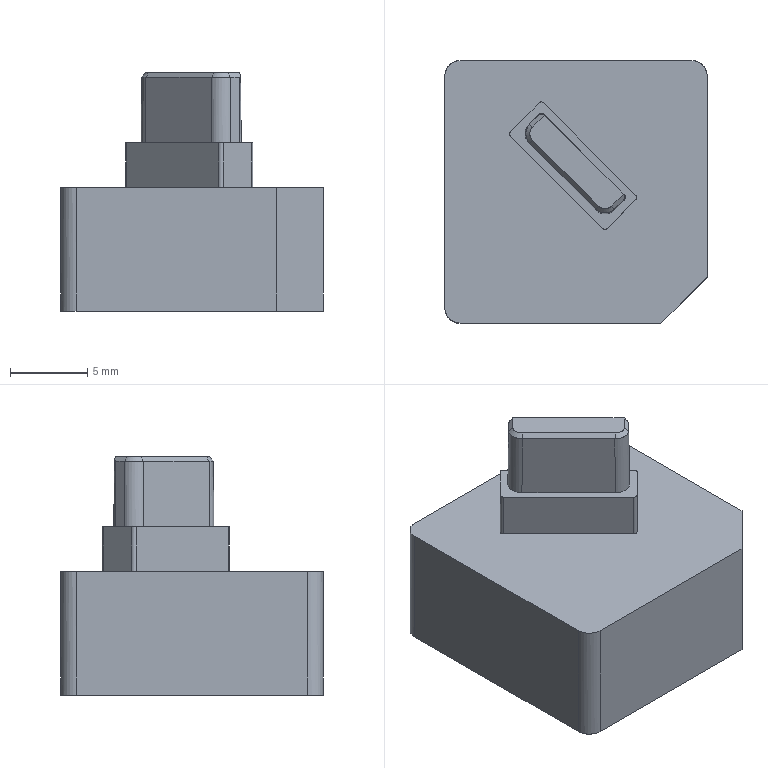NC program | PowerMill | posted with a generic post | part box 17 x 17 x 15.424 mm
Lines 1 to 1056 of 24748:
%
O0001
N104 ( POWERMILL CB  : 2026004.0)
N105 ( POST VER      : 2026.0.0.5161)
N106 ( OPTION FILE   : FANUC)
N107 ( OUTPUT WORKPLANE : WORLD)
N108 (  )
N109 ( TOOL LIST )
N110 (---------------------------------------)
N111 ( NO. | ID        | DIA.| TIP RAD|LENGTH)
N112 (---------------------------------------)
N113 (    1|D10C_1_1   |10.0 |  0.0   |70.88 )
N114 (    3|D10_1_1    |10.0 |  0.0   | 70.6 )
N115 (   14|D4_2_1     | 4.0 |  0.0   |62.44 )
N116 (   13|TEXT_D4_1_1| 4.0 |  0.3   |62.68 )
N117 (---------------------------------------)
N118 (  )
N119 ( NUMBER OF TOOLPATHS: 10.0 )
N120 ( ESTIMATED PROGRAM DURATION: 0 HOURS 3 MIN 55 SEC)
N121 (  )
N122 G00 G21 G80 G40 G17
N123 G90
N124 G54
N125 G53 Z0.0
N126 (---------------)
N127 ( START TOOLPATH : 粗公开粗01-扫面平行-D10C )
N128 (---------------)
N129 ( TOOL NO.    :1 )
N130 ( TOOL TYPE   : ENDMILL)
N131 ( TOOL ID     : D10C_1_1)
N132 ( TOOL DIA    : 10.0 LENGTH 70.88)
N133 T1
N134 M6
N135 S8000 M03
N136 G00 G90 X0.0 Y0.0
N137 G43 Z10.2 H1
N138
N139 G05 P10000 R4
N140 X16.15 Y11.15
N141 Z1.004
N142 G01 Z-0.196 F6000.0
N143 X11.15 F10000.0
N144 X-11.15
N145 Y5.575
N146 X11.15
N147 Y0.0
N148 X-11.15
N149 Y-5.575
N150 X11.15
N151 Y-11.15
N152 X-11.15
N153 X-16.15
N154 G00 Z10.2
N155 G05 P0
N156 (---------------)
N157 ( END TOOLPATH : 粗公开粗01-扫面平行-D10C )
N158 (---------------)
N159 ( START TOOLPATH : 粗公开粗01-外形偏置-D10C )
N160 (---------------)
N161 G00 X-0.181 Y1.1575 Z9.8043
N162 G05 P10000 R4
N163 X16.863 Y4.7263
N164 Z0.5804
N165 G01 Z-0.6196 F6000.0
N166 X16.3355 F10000.0
N167 G03 X11.588 Y-0.0212 I0.0 J-4.7475
N168 G01 Y-10.15
N169 G02 X10.588 Y-11.15 I-1.0 J0.0
N170 G01 X-10.95
N171 G02 X-11.95 Y-10.15 I0.0 J1.0
N172 G01 Y12.465
N173 G02 X-10.95 Y13.465 I1.0 J0.0
N174 G01 X10.588
N175 G02 X11.588 Y12.465 I0.0 J-1.0
N176 G01 Y-0.0212
N177 X8.2778 Y-0.0026
N178 X8.2734 Y-0.7761
N179 X8.1572 Y-1.5495
N180 X7.9222 Y-2.3229
N181 X7.5545 Y-3.0963
N182 X7.0126 Y-3.8698
N183 X6.7798 Y-4.1306
N184 X6.0064 Y-4.9002
N185 X5.3694 Y-5.4166
N186 X4.4596 Y-5.9486
N187 X3.8629 Y-6.1901
N188 X2.9127 Y-6.4361
N189 X2.1393 Y-6.5083
N190 X1.3659 Y-6.4953
N191 X0.5924 Y-6.386
N192 X-0.1057 Y-6.1901
N193 X-0.9544 Y-5.8196
N194 X-1.6123 Y-5.4166
N195 X-2.5116 Y-4.6432
N196 X-6.3782 Y-0.7761
N197 X-7.0949 Y-0.0026
N198 X-7.616 Y0.7708
N199 X-7.9153 Y1.3758
N200 X-8.2299 Y2.3176
N201 X-8.3654 Y3.0911
N202 X-8.4023 Y3.8645
N203 X-8.3373 Y4.6379
N204 X-8.1726 Y5.4113
N205 X-7.9153 Y6.137
N206 X-7.4873 Y6.9582
N207 X-7.1418 Y7.4555
N208 X-6.9153 Y7.7316
N209 X-6.1617 Y8.5051
N210 X-5.595 Y9.0122
N211 X-5.2191 Y9.2785
N212 X-4.8216 Y9.5163
N213 X-4.0481 Y9.8551
N214 X-3.3652 Y10.0519
N215 X-2.5013 Y10.1631
N216 X-1.7279 Y10.1418
N217 X-1.1171 Y10.0519
N218 X-0.181 Y9.7628
N219 X0.5924 Y9.3654
N220 X1.3659 Y8.8028
N221 X1.6815 Y8.5051
N222 X6.7798 Y3.4047
N223 X7.0556 Y3.0911
N224 X7.5533 Y2.3604
N225 X7.9456 Y1.5442
N226 X8.1721 Y0.7708
N227 X8.2778 Y-0.0026
N228 X11.588 Y-0.0212
N229 G00 Z3.2568
N230 G01 X16.863 Y4.7263
N231 G00 Z0.2068
N232 G01 Z-0.9932 F6000.0
N233 X16.3355 F10000.0
N234 G03 X11.588 Y-0.0212 I0.0 J-4.7475
N235 G01 Y-10.15
N236 G02 X10.588 Y-11.15 I-1.0 J0.0
N237 G01 X-10.95
N238 G02 X-11.95 Y-10.15 I0.0 J1.0
N239 G01 Y12.465
N240 G02 X-10.95 Y13.465 I1.0 J0.0
N241 G01 X10.588
N242 G02 X11.588 Y12.465 I0.0 J-1.0
N243 G01 Y-0.0184
N244 X8.2821 Y-0.0026
N245 X8.2784 Y-0.7761
N246 X8.1655 Y-1.5495
N247 X7.9286 Y-2.3229
N248 X7.5585 Y-3.0963
N249 X7.0174 Y-3.8698
N250 X6.7798 Y-4.1361
N251 X6.0064 Y-4.9058
N252 X5.3695 Y-5.4166
N253 X4.4596 Y-5.9532
N254 X3.863 Y-6.1901
N255 X2.9127 Y-6.4424
N256 X2.1393 Y-6.518
N257 X1.3659 Y-6.5069
N258 X0.5924 Y-6.3915
N259 X-0.1057 Y-6.1901
N260 X-0.9544 Y-5.8258
N261 X-1.6125 Y-5.4166
N262 X-2.5173 Y-4.6432
N263 X-6.3844 Y-0.7761
N264 X-7.0951 Y-0.0026
N265 X-7.6206 Y0.7708
N266 X-7.9153 Y1.3672
N267 X-8.232 Y2.3176
N268 X-8.3713 Y3.0911
N269 X-8.4027 Y3.8645
N270 X-8.3446 Y4.6379
N271 X-8.1727 Y5.4113
N272 X-7.9153 Y6.1457
N273 X-7.4886 Y6.9582
N274 X-7.1418 Y7.4556
N275 X-6.9197 Y7.7316
N276 X-6.3684 Y8.303
N277 X-6.2691 Y8.3947
N278 X-6.1616 Y8.505
N279 X-5.7765 Y8.8497
N280 X-5.595 Y9.0173
N281 X-5.2267 Y9.2785
N282 X-4.8216 Y9.5221
N283 X-4.0481 Y9.865
N284 X-3.3869 Y10.0519
N285 X-2.5013 Y10.1671
N286 X-1.7279 Y10.1457
N287 X-1.0956 Y10.0519
N288 X-0.181 Y9.7672
N289 X0.5924 Y9.3694
N290 X1.3659 Y8.8095
N291 X1.6861 Y8.5051
N292 X6.7798 Y3.4095
N293 X7.0602 Y3.0911
N294 X7.5533 Y2.364
N295 X7.9502 Y1.5442
N296 X8.1767 Y0.7708
N297 X8.2821 Y-0.0026
N298 X11.588 Y-0.0184
N299 Y-0.0212
N300 G00 Z2.8832
N301 G01 X16.863 Y4.7263
N302 G00 Z-0.1668
N303 G01 Z-1.3668 F6000.0
N304 X16.3355 F10000.0
N305 G03 X11.588 Y-0.0212 I0.0 J-4.7475
N306 G01 Y-0.0233
N307 X8.2864 Y-0.0026
N308 X8.2815 Y-0.7761
N309 X8.1701 Y-1.5495
N310 X7.9347 Y-2.3229
N311 X7.5623 Y-3.0963
N312 X7.022 Y-3.8698
N313 X6.7798 Y-4.1409
N314 X6.0064 Y-4.9104
N315 X5.3695 Y-5.4166
N316 X4.4596 Y-5.9578
N317 X3.8663 Y-6.1901
N318 X2.9127 Y-6.447
N319 X2.1393 Y-6.5236
N320 X1.3659 Y-6.5115
N321 X0.5924 Y-6.3961
N322 X-0.109 Y-6.1901
N323 X-0.9544 Y-5.832
N324 X-1.6128 Y-5.4166
N325 X-2.5013 Y-4.6638
N326 X-6.389 Y-0.7761
N327 X-7.0994 Y-0.0026
N328 X-7.6252 Y0.7708
N329 X-7.9153 Y1.3565
N330 X-8.2366 Y2.3176
N331 X-8.376 Y3.0911
N332 X-8.4031 Y3.8645
N333 X-8.3492 Y4.6379
N334 X-8.1753 Y5.4113
N335 X-7.9035 Y6.1848
N336 X-7.4932 Y6.9582
N337 X-7.4041 Y7.0793
N338 X-7.1418 Y7.4555
N339 X-6.9722 Y7.6663
N340 X-6.9242 Y7.7316
N341 X-6.3684 Y8.3095
N342 X-6.2093 Y8.456
N343 X-6.1616 Y8.505
N344 X-5.9709 Y8.6756
N345 X-5.595 Y9.0219
N346 X-5.2334 Y9.2785
N347 X-4.8216 Y9.5255
N348 X-4.0481 Y9.8696
N349 X-3.4086 Y10.0519
N350 X-2.5013 Y10.1711
N351 X-1.7279 Y10.1501
N352 X-1.0742 Y10.0519
N353 X-0.181 Y9.7718
N354 X0.5924 Y9.374
N355 X1.3659 Y8.8141
N356 X1.6907 Y8.5051
N357 X6.7798 Y3.4143
N358 X7.0648 Y3.0911
N359 X7.5533 Y2.372
N360 X7.9548 Y1.5442
N361 X8.1813 Y0.7708
N362 X8.2864 Y-0.0026
N363 X11.588 Y-0.0233
N364 Y-10.15
N365 G02 X10.588 Y-11.15 I-1.0 J0.0
N366 G01 X-10.95
N367 G02 X-11.95 Y-10.15 I0.0 J1.0
N368 G01 Y12.465
N369 G02 X-10.95 Y13.465 I1.0 J0.0
N370 G01 X10.588
N371 G02 X11.588 Y12.465 I0.0 J-1.0
N372 G01 Y-0.0212
N373 G00 Z2.5096
N374 G01 X16.863 Y4.7263
N375 G00 Z-0.5404
N376 G01 Z-1.7404 F6000.0
N377 X16.3355 F10000.0
N378 G03 X11.588 Y-0.0212 I0.0 J-4.7475
N379 G01 Y-0.0276
N380 X8.2907 Y-0.0026
N381 X8.2848 Y-0.7761
N382 X8.1747 Y-1.5495
N383 X7.9393 Y-2.3229
N384 X7.5661 Y-3.0963
N385 X7.0267 Y-3.8698
N386 X6.7798 Y-4.1457
N387 X6.0064 Y-4.915
N388 X5.3744 Y-5.4166
N389 X4.4596 Y-5.9624
N390 X3.88 Y-6.1901
N391 X2.9127 Y-6.4516
N392 X2.1393 Y-6.5282
N393 X1.3659 Y-6.5161
N394 X0.5924 Y-6.4007
N395 X-0.181 Y-6.1709
N396 X-0.9544 Y-5.8367
N397 X-1.6172 Y-5.4166
N398 X-2.5013 Y-4.6684
N399 X-6.3684 Y-0.8013
N400 X-7.1037 Y-0.0026
N401 X-7.6298 Y0.7708
N402 X-7.9153 Y1.3457
N403 X-8.2412 Y2.3176
N404 X-8.3806 Y3.0911
N405 X-8.4073 Y3.8645
N406 X-8.3539 Y4.6379
N407 X-8.1799 Y5.4113
N408 X-7.9153 Y6.1677
N409 X-7.4978 Y6.9582
N410 X-7.3205 Y7.199
N411 X-7.1418 Y7.4555
N412 X-7.0251 Y7.6005
N413 X-6.9286 Y7.7316
N414 X-6.3684 Y8.3141
N415 X-6.1647 Y8.5017
N416 X-6.1616 Y8.5049
N417 X-6.1489 Y8.5163
N418 X-5.595 Y9.0265
N419 X-5.2401 Y9.2785
N420 X-4.8216 Y9.529
N421 X-4.0481 Y9.8742
N422 X-3.4294 Y10.0519
N423 X-2.5013 Y10.1751
N424 X-1.7279 Y10.1547
N425 X-1.0527 Y10.0519
N426 X-0.181 Y9.7764
N427 X0.5924 Y9.3786
N428 X1.3659 Y8.8187
N429 X1.6953 Y8.5051
N430 X6.7798 Y3.4191
N431 X7.0694 Y3.0911
N432 X7.5533 Y2.38
N433 X7.9594 Y1.5442
N434 X8.1859 Y0.7708
N435 X8.2907 Y-0.0026
N436 X11.588 Y-0.0276
N437 Y-10.15
N438 G02 X10.588 Y-11.15 I-1.0 J0.0
N439 G01 X-10.95
N440 G02 X-11.95 Y-10.15 I0.0 J1.0
N441 G01 Y12.465
N442 G02 X-10.95 Y13.465 I1.0 J0.0
N443 G01 X10.588
N444 G02 X11.588 Y12.465 I0.0 J-1.0
N445 G01 Y-0.0212
N446 G00 Z2.136
N447 G01 X16.863 Y4.7263
N448 G00 Z-0.914
N449 G01 Z-2.114 F6000.0
N450 X16.3355 F10000.0
N451 G03 X11.588 Y-0.0212 I0.0 J-4.7475
N452 G01 Y-0.0276
N453 X8.2949 Y-0.0026
N454 X8.2891 Y-0.7761
N455 X8.1793 Y-1.5495
N456 X7.9439 Y-2.3229
N457 X7.5699 Y-3.0963
N458 X7.0313 Y-3.8698
N459 X6.7798 Y-4.1505
N460 X6.0064 Y-4.9195
N461 X5.6851 Y-5.1699
N462 X5.3744 Y-5.4166
N463 X5.35 Y-5.4311
N464 X5.233 Y-5.5223
N465 X4.4596 Y-5.967
N466 X3.8938 Y-6.1901
N467 X2.9127 Y-6.4562
N468 X2.1393 Y-6.5328
N469 X1.3659 Y-6.5207
N470 X0.5924 Y-6.4053
N471 X-0.181 Y-6.1755
N472 X-0.9544 Y-5.8414
N473 X-1.6231 Y-5.4166
N474 X-2.5013 Y-4.673
N475 X-6.3684 Y-0.8059
N476 X-7.108 Y-0.0026
N477 X-7.6344 Y0.7708
N478 X-7.9153 Y1.3349
N479 X-8.2458 Y2.3176
N480 X-8.3852 Y3.0911
N481 X-8.4119 Y3.8645
N482 X-8.3585 Y4.6379
N483 X-8.1845 Y5.4113
N484 X-7.9153 Y6.1787
N485 X-7.5024 Y6.9582
N486 X-7.238 Y7.3173
N487 X-7.1417 Y7.4555
N488 X-7.0783 Y7.5343
N489 X-6.933 Y7.7316
N490 X-6.3684 Y8.3187
N491 X-5.595 Y9.0311
N492 X-5.2468 Y9.2785
N493 X-4.8216 Y9.5324
N494 X-4.0481 Y9.8788
N495 X-3.4497 Y10.0519
N496 X-2.5013 Y10.1791
N497 X-1.7279 Y10.1593
N498 X-1.0318 Y10.0519
N499 X-0.181 Y9.781
N500 X0.5924 Y9.3833
N501 X1.3659 Y8.8233
N502 X1.6999 Y8.5051
N503 X6.7798 Y3.4239
N504 X7.0741 Y3.0911
N505 X7.5533 Y2.3879
N506 X7.9641 Y1.5442
N507 X8.1905 Y0.7708
N508 X8.2949 Y-0.0026
N509 X11.588 Y-0.0276
N510 Y-10.15
N511 G02 X10.588 Y-11.15 I-1.0 J0.0
N512 G01 X-10.95
N513 G02 X-11.95 Y-10.15 I0.0 J1.0
N514 G01 Y12.465
N515 G02 X-10.95 Y13.465 I1.0 J0.0
N516 G01 X10.588
N517 G02 X11.588 Y12.465 I0.0 J-1.0
N518 G01 Y-0.0212
N519 G00 Z1.7624
N520 G01 X16.863 Y4.7263
N521 G00 Z-1.2876
N522 G01 Z-2.4876 F6000.0
N523 X16.3355 F10000.0
N524 G03 X11.588 Y-0.0212 I0.0 J-4.7475
N525 G01 Y-0.0261
N526 X8.2992 Y-0.0026
N527 X8.2937 Y-0.7761
N528 X8.1839 Y-1.5495
N529 X7.9485 Y-2.3229
N530 X7.5736 Y-3.0963
N531 X7.0359 Y-3.8698
N532 X6.7798 Y-4.1553
N533 X6.0064 Y-4.924
N534 X5.233 Y-5.5269
N535 X4.4596 Y-5.9716
N536 X3.9076 Y-6.1901
N537 X2.9127 Y-6.4608
N538 X2.1393 Y-6.5374
N539 X1.3659 Y-6.5254
N540 X0.5924 Y-6.4099
N541 X-0.181 Y-6.1802
N542 X-0.9544 Y-5.846
N543 X-1.6293 Y-5.4166
N544 X-2.5013 Y-4.6777
N545 X-6.4029 Y-0.7761
N546 X-7.1123 Y-0.0026
N547 X-7.6391 Y0.7708
N548 X-7.9153 Y1.3242
N549 X-8.2505 Y2.3176
N550 X-8.3898 Y3.0911
N551 X-8.4165 Y3.8645
N552 X-8.3631 Y4.6379
N553 X-8.1891 Y5.4113
N554 X-7.9173 Y6.1848
N555 X-7.507 Y6.9582
N556 X-7.1565 Y7.4342
N557 X-7.1417 Y7.4554
N558 X-7.1318 Y7.4677
N559 X-6.9375 Y7.7316
N560 X-6.3684 Y8.3233
N561 X-5.595 Y9.0357
N562 X-5.2535 Y9.2785
N563 X-4.8216 Y9.5358
N564 X-4.0481 Y9.8834
N565 X-3.47 Y10.0519
N566 X-2.5013 Y10.1831
N567 X-1.7279 Y10.1639
N568 X-1.012 Y10.0519
N569 X-0.181 Y9.7857
N570 X0.0594 Y9.6573
N571 X0.5924 Y9.3832
N572 X0.6468 Y9.3438
N573 X0.7692 Y9.2785
N574 X1.3659 Y8.8279
N575 X1.7045 Y8.5051
N576 X6.7798 Y3.4287
N577 X7.0787 Y3.0911
N578 X7.5533 Y2.3959
N579 X7.9687 Y1.5442
N580 X8.1951 Y0.7708
N581 X8.2992 Y-0.0026
N582 X11.588 Y-0.0261
N583 Y-10.15
N584 G02 X10.588 Y-11.15 I-1.0 J0.0
N585 G01 X-10.95
N586 G02 X-11.95 Y-10.15 I0.0 J1.0
N587 G01 Y12.465
N588 G02 X-10.95 Y13.465 I1.0 J0.0
N589 G01 X10.588
N590 G02 X11.588 Y12.465 I0.0 J-1.0
N591 G01 Y-0.0212
N592 G00 Z1.3888
N593 G01 X16.863 Y4.7263
N594 G00 Z-1.6612
N595 G01 Z-2.8612 F6000.0
N596 X16.3355 F10000.0
N597 G03 X11.588 Y-0.0212 I0.0 J-4.7475
N598 G01 Y-0.0245
N599 X8.3035 Y-0.0026
N600 X8.2983 Y-0.7761
N601 X8.1885 Y-1.5495
N602 X7.9531 Y-2.3229
N603 X7.5773 Y-3.0963
N604 X7.0405 Y-3.8698
N605 X6.7798 Y-4.16
N606 X6.0064 Y-4.9286
N607 X5.233 Y-5.5316
N608 X4.4596 Y-5.9762
N609 X3.9214 Y-6.1901
N610 X2.9127 Y-6.4654
N611 X2.1393 Y-6.542
N612 X1.3659 Y-6.53
N613 X0.5924 Y-6.4145
N614 X-0.164 Y-6.1901
N615 X-0.9544 Y-5.8506
N616 X-1.6357 Y-5.4166
N617 X-2.5013 Y-4.6823
N618 X-6.4075 Y-0.7761
N619 X-7.1166 Y-0.0026
N620 X-7.6437 Y0.7708
N621 X-7.9153 Y1.3134
N622 X-8.2551 Y2.3176
N623 X-8.3944 Y3.0911
N624 X-8.4212 Y3.8645
N625 X-8.3677 Y4.6379
N626 X-8.1937 Y5.4113
N627 X-7.9219 Y6.1848
N628 X-7.5116 Y6.9582
N629 X-6.9419 Y7.7316
N630 X-6.3684 Y8.3279
N631 X-5.595 Y9.0403
N632 X-5.2602 Y9.2785
N633 X-4.8216 Y9.5391
N634 X-4.0481 Y9.888
N635 X-3.8216 Y9.9494
N636 X-3.47 Y10.0519
N637 X-3.4166 Y10.0591
N638 X-3.2747 Y10.0975
N639 X-2.5013 Y10.187
N640 X-1.7279 Y10.1685
N641 X-0.9922 Y10.0519
N642 X-0.181 Y9.7903
N643 X0.2797 Y9.544
N644 X0.5924 Y9.3832
N645 X0.6258 Y9.3589
N646 X0.7764 Y9.2785
N647 X1.3659 Y8.8325
N648 X1.7091 Y8.5051
N649 X6.7798 Y3.4334
N650 X7.0833 Y3.0911
N651 X7.5533 Y2.4039
N652 X7.9733 Y1.5442
N653 X8.1997 Y0.7708
N654 X8.3035 Y-0.0026
N655 X11.588 Y-0.0245
N656 Y-10.15
N657 G02 X10.588 Y-11.15 I-1.0 J0.0
N658 G01 X-10.95
N659 G02 X-11.95 Y-10.15 I0.0 J1.0
N660 G01 Y12.465
N661 G02 X-10.95 Y13.465 I1.0 J0.0
N662 G01 X10.588
N663 G02 X11.588 Y12.465 I0.0 J-1.0
N664 G01 Y-0.0212
N665 G00 Z1.0152
N666 G01 X16.863 Y4.7263
N667 G00 Z-2.0348
N668 G01 Z-3.2348 F6000.0
N669 X16.3355 F10000.0
N670 G03 X11.588 Y-0.0212 I0.0 J-4.7475
N671 G01 Y-0.0229
N672 X8.3077 Y-0.0026
N673 X8.3029 Y-0.7761
N674 X8.1932 Y-1.5495
N675 X7.9577 Y-2.3229
N676 X7.581 Y-3.0963
N677 X7.0451 Y-3.8698
N678 X6.7798 Y-4.1648
N679 X6.0064 Y-4.9331
N680 X5.233 Y-5.5362
N681 X4.4596 Y-5.9808
N682 X3.9351 Y-6.1901
N683 X2.9127 Y-6.47
N684 X2.1393 Y-6.5466
N685 X1.3659 Y-6.5346
N686 X0.5924 Y-6.4191
N687 X-0.181 Y-6.1894
N688 X-0.9544 Y-5.8552
N689 X-1.642 Y-5.4166
N690 X-2.5013 Y-4.6869
N691 X-6.4121 Y-0.7761
N692 X-7.1209 Y-0.0026
N693 X-7.6483 Y0.7708
N694 X-7.9153 Y1.3027
N695 X-8.2597 Y2.3176
N696 X-8.399 Y3.0911
N697 X-8.4258 Y3.8645
N698 X-8.3723 Y4.6379
N699 X-8.1983 Y5.4113
N700 X-7.9265 Y6.1848
N701 X-7.5162 Y6.9582
N702 X-6.9463 Y7.7316
N703 X-6.3684 Y8.3325
N704 X-5.595 Y9.045
N705 X-5.2669 Y9.2785
N706 X-4.8216 Y9.5427
N707 X-4.0481 Y9.8926
N708 X-3.5949 Y10.0154
N709 X-3.47 Y10.0518
N710 X-3.451 Y10.0544
N711 X-3.2747 Y10.1021
N712 X-2.5013 Y10.191
N713 X-1.7279 Y10.1732
N714 X-0.9723 Y10.0519
N715 X-0.181 Y9.7949
N716 X0.4821 Y9.4398
N717 X0.5923 Y9.3831
N718 X0.6047 Y9.3742
N719 X0.7834 Y9.2785
N720 X1.3659 Y8.8371
N721 X1.7137 Y8.5051
N722 X6.7798 Y3.4382
N723 X7.0879 Y3.0911
N724 X7.5533 Y2.4119
N725 X7.9779 Y1.5442
N726 X8.2044 Y0.7708
N727 X8.3077 Y-0.0026
N728 X11.588 Y-0.0229
N729 Y-10.15
N730 G02 X10.588 Y-11.15 I-1.0 J0.0
N731 G01 X-10.95
N732 G02 X-11.95 Y-10.15 I0.0 J1.0
N733 G01 Y12.465
N734 G02 X-10.95 Y13.465 I1.0 J0.0
N735 G01 X10.588
N736 G02 X11.588 Y12.465 I0.0 J-1.0
N737 G01 Y-0.0212
N738 G00 Z0.6416
N739 G01 X16.863 Y4.7263
N740 G00 Z-2.4084
N741 G01 Z-3.6084 F6000.0
N742 X16.3355 F10000.0
N743 G03 X11.588 Y-0.0212 I0.0 J-4.7475
N744 G01 Y-0.0213
N745 X8.3119 Y-0.0026
N746 X8.3075 Y-0.7761
N747 X8.1978 Y-1.5495
N748 X7.9624 Y-2.3229
N749 X7.5847 Y-3.0963
N750 X7.0497 Y-3.8698
N751 X6.7798 Y-4.1695
N752 X6.0064 Y-4.9376
N753 X5.233 Y-5.5408
N754 X4.4596 Y-5.9854
N755 X3.9489 Y-6.1901
N756 X2.9127 Y-6.4746
N757 X2.1393 Y-6.5512
N758 X1.3659 Y-6.5392
N759 X0.5924 Y-6.4238
N760 X-0.181 Y-6.194
N761 X-0.9544 Y-5.8598
N762 X-1.6484 Y-5.4166
N763 X-2.2585 Y-4.893
N764 X-2.5012 Y-4.6868
N765 X-2.5166 Y-4.6715
N766 X-2.5496 Y-4.6432
N767 X-6.4167 Y-0.7761
N768 X-7.1252 Y-0.0026
N769 X-7.6529 Y0.7708
N770 X-7.9153 Y1.2919
N771 X-8.0175 Y1.5442
N772 X-8.2643 Y2.3176
N773 X-8.4037 Y3.0911
N774 X-8.4304 Y3.8645
N775 X-8.3769 Y4.6379
N776 X-8.2029 Y5.4113
N777 X-7.9311 Y6.1848
N778 X-7.5209 Y6.9582
N779 X-6.9508 Y7.7316
N780 X-6.3684 Y8.3371
N781 X-5.595 Y9.0496
N782 X-5.2736 Y9.2785
N783 X-4.8216 Y9.5473
N784 X-4.0481 Y9.8972
N785 X-3.2747 Y10.1067
N786 X-2.5013 Y10.195
N787 X-1.7279 Y10.1778
N788 X-0.9544 Y10.0524
N789 X-0.181 Y9.7995
N790 X0.7905 Y9.2785
N791 X1.3659 Y8.8417
N792 X1.7184 Y8.5051
N793 X6.7798 Y3.4429
N794 X7.0925 Y3.0911
N795 X7.5533 Y2.4198
N796 X7.9825 Y1.5442
N797 X8.209 Y0.7708
N798 X8.3119 Y-0.0026
N799 X11.588 Y-0.0213
N800 Y-10.15
N801 G02 X10.588 Y-11.15 I-1.0 J0.0
N802 G01 X-10.95
N803 G02 X-11.95 Y-10.15 I0.0 J1.0
N804 G01 Y12.465
N805 G02 X-10.95 Y13.465 I1.0 J0.0
N806 G01 X10.588
N807 G02 X11.588 Y12.465 I0.0 J-1.0
N808 G01 Y-0.0212
N809 G00 Z0.268
N810 G01 X16.863 Y4.7263
N811 G00 Z-2.782
N812 G01 Z-3.982 F6000.0
N813 X16.3355 F10000.0
N814 G03 X11.588 Y-0.0212 I0.0 J-4.7475
N815 G01 Y-10.15
N816 G02 X10.588 Y-11.15 I-1.0 J0.0
N817 G01 X-10.95
N818 G02 X-11.95 Y-10.15 I0.0 J1.0
N819 G01 Y12.465
N820 G02 X-10.95 Y13.465 I1.0 J0.0
N821 G01 X10.588
N822 G02 X11.588 Y12.465 I0.0 J-1.0
N823 G01 Y-0.0195
N824 X8.3161 Y-0.0026
N825 X8.3121 Y-0.7761
N826 X8.2024 Y-1.5495
N827 X7.967 Y-2.3229
N828 X7.5884 Y-3.0963
N829 X7.0543 Y-3.8698
N830 X6.7798 Y-4.1742
N831 X6.0064 Y-4.9422
N832 X5.233 Y-5.5454
N833 X4.4596 Y-5.9901
N834 X3.9627 Y-6.1901
N835 X2.9127 Y-6.4793
N836 X2.1393 Y-6.5558
N837 X1.3659 Y-6.5438
N838 X0.5924 Y-6.4284
N839 X-0.181 Y-6.1986
N840 X-0.9544 Y-5.8644
N841 X-1.6547 Y-5.4166
N842 X-2.5542 Y-4.6432
N843 X-6.4213 Y-0.7761
N844 X-7.1295 Y-0.0026
N845 X-7.6575 Y0.7708
N846 X-7.9153 Y1.2812
N847 X-8.0221 Y1.5442
N848 X-8.2689 Y2.3176
N849 X-8.4083 Y3.0911
N850 X-8.435 Y3.8645
N851 X-8.3815 Y4.6379
N852 X-8.2076 Y5.4113
N853 X-7.9358 Y6.1848
N854 X-7.5255 Y6.9582
N855 X-6.9552 Y7.7316
N856 X-6.3684 Y8.3417
N857 X-5.595 Y9.0542
N858 X-5.2803 Y9.2785
N859 X-4.8216 Y9.5519
N860 X-4.0481 Y9.9019
N861 X-3.2747 Y10.1114
N862 X-2.5013 Y10.1989
N863 X-1.7279 Y10.1824
N864 X-0.9544 Y10.057
N865 X-0.181 Y9.8041
N866 X0.5924 Y9.4063
N867 X0.7975 Y9.2785
N868 X1.3659 Y8.8463
N869 X1.723 Y8.5051
N870 X6.7798 Y3.4477
N871 X7.0971 Y3.0911
N872 X7.5533 Y2.4278
N873 X7.9871 Y1.5442
N874 X8.2136 Y0.7708
N875 X8.3161 Y-0.0026
N876 X11.588 Y-0.0195
N877 Y-0.0212
N878 G00 Z-0.1056
N879 G01 X16.863 Y4.7263
N880 G00 Z-3.1556
N881 G01 Z-4.3556 F6000.0
N882 X16.3355 F10000.0
N883 G03 X11.588 Y-0.0212 I0.0 J-4.7475
N884 G01 Y-10.15
N885 G02 X10.588 Y-11.15 I-1.0 J0.0
N886 G01 X-10.95
N887 G02 X-11.95 Y-10.15 I0.0 J1.0
N888 G01 Y12.465
N889 G02 X-10.95 Y13.465 I1.0 J0.0
N890 G01 X10.588
N891 G02 X11.588 Y12.465 I0.0 J-1.0
N892 G01 Y-0.0178
N893 X8.3203 Y-0.0026
N894 X8.3167 Y-0.7761
N895 X8.207 Y-1.5495
N896 X7.9716 Y-2.3229
N897 X7.592 Y-3.0963
N898 X7.0589 Y-3.8698
N899 X6.7798 Y-4.179
N900 X6.0064 Y-4.9467
N901 X5.233 Y-5.55
N902 X4.4596 Y-5.9947
N903 X3.9764 Y-6.1901
N904 X2.9127 Y-6.4839
N905 X2.1393 Y-6.5604
N906 X1.3659 Y-6.5484
N907 X0.5924 Y-6.433
N908 X-0.219 Y-6.1901
N909 X-0.9544 Y-5.869
N910 X-1.6611 Y-5.4166
N911 X-2.5013 Y-4.7007
N912 X-6.4259 Y-0.7761
N913 X-7.1338 Y-0.0026
N914 X-7.6621 Y0.7708
N915 X-7.9153 Y1.2704
N916 X-8.0267 Y1.5442
N917 X-8.2735 Y2.3176
N918 X-8.4129 Y3.0911
N919 X-8.4396 Y3.8645
N920 X-8.3861 Y4.6379
N921 X-8.2122 Y5.4113
N922 X-7.9404 Y6.1848
N923 X-7.5301 Y6.9582
N924 X-6.9596 Y7.7316
N925 X-6.3684 Y8.3463
N926 X-5.595 Y9.0588
N927 X-5.287 Y9.2785
N928 X-4.8216 Y9.5565
N929 X-4.0481 Y9.9065
N930 X-3.2747 Y10.116
N931 X-2.5013 Y10.2029
N932 X-1.7279 Y10.187
N933 X-0.9544 Y10.0616
N934 X-0.181 Y9.8087
N935 X0.5924 Y9.4109
N936 X0.8046 Y9.2785
N937 X1.3659 Y8.851
N938 X1.7276 Y8.5051
N939 X6.7798 Y3.4524
N940 X7.1017 Y3.0911
N941 X7.5533 Y2.4358
N942 X7.9917 Y1.5442
N943 X8.2182 Y0.7708
N944 X8.3203 Y-0.0026
N945 X11.588 Y-0.0178
N946 Y-0.0212
N947 G00 Z-0.4792
N948 G01 X16.863 Y4.7263
N949 G00 Z-3.5292
N950 G01 Z-4.7292 F6000.0
N951 X16.3355 F10000.0
N952 G03 X11.588 Y-0.0212 I0.0 J-4.7475
N953 G01 Y-10.15
N954 G02 X10.588 Y-11.15 I-1.0 J0.0
N955 G01 X-10.95
N956 G02 X-11.95 Y-10.15 I0.0 J1.0
N957 G01 Y12.465
N958 G02 X-10.95 Y13.465 I1.0 J0.0
N959 G01 X10.588
N960 G02 X11.588 Y12.465 I0.0 J-1.0
N961 G01 Y0.0078
N962 X8.3245 Y-0.0026
N963 X8.3267 Y-0.6797
N964 X8.3168 Y-0.7546
N965 X8.3167 Y-0.7761
N966 X8.276 Y-1.0628
N967 X8.2116 Y-1.5495
N968 X7.9762 Y-2.3229
N969 X7.596 Y-3.0963
N970 X7.0635 Y-3.8698
N971 X6.7798 Y-4.1837
N972 X6.0064 Y-4.9512
N973 X5.233 Y-5.5546
N974 X4.4596 Y-5.9993
N975 X3.9902 Y-6.1901
N976 X3.6861 Y-6.2901
N977 X2.9127 Y-6.4885
N978 X2.1393 Y-6.565
N979 X1.3659 Y-6.553
N980 X0.5924 Y-6.4376
N981 X-0.2328 Y-6.1901
N982 X-0.9544 Y-5.8736
N983 X-1.6674 Y-5.4166
N984 X-2.5013 Y-4.7053
N985 X-6.4305 Y-0.7761
N986 X-7.1381 Y-0.0026
N987 X-7.6667 Y0.7708
N988 X-7.9153 Y1.2596
N989 X-8.0313 Y1.5442
N990 X-8.2781 Y2.3176
N991 X-8.4175 Y3.0911
N992 X-8.4442 Y3.8645
N993 X-8.3907 Y4.6379
N994 X-8.2168 Y5.4113
N995 X-7.945 Y6.1848
N996 X-7.5347 Y6.9582
N997 X-6.964 Y7.7316
N998 X-6.3684 Y8.351
N999 X-5.595 Y9.0634
N1000 X-5.2937 Y9.2785
N1001 X-4.8216 Y9.5611
N1002 X-4.0481 Y9.9111
N1003 X-3.2747 Y10.1206
N1004 X-2.5013 Y10.2068
N1005 X-1.7279 Y10.1916
N1006 X-0.9544 Y10.0662
N1007 X-0.181 Y9.8133
N1008 X0.5924 Y9.4155
N1009 X0.8116 Y9.2785
N1010 X1.3659 Y8.8556
N1011 X1.7322 Y8.5051
N1012 X6.7798 Y3.4571
N1013 X7.1063 Y3.0911
N1014 X7.5533 Y2.4438
N1015 X7.9963 Y1.5442
N1016 X8.2228 Y0.7708
N1017 X8.3245 Y-0.0026
N1018 X11.588 Y0.0078
N1019 Y-0.0212
N1020 G00 Z-0.8707
N1021 G01 X16.863 Y4.7263
N1022 G00 Z-3.9207
N1023 G01 Z-5.1207 F6000.0
N1024 X16.3355 F10000.0
N1025 G03 X11.588 Y-0.0212 I0.0 J-4.7475
N1026 G01 Y-10.15
N1027 G02 X10.588 Y-11.15 I-1.0 J0.0
N1028 G01 X-10.95
N1029 G02 X-11.95 Y-10.15 I0.0 J1.0
N1030 G01 Y3.553
N1031 X-9.4382 Y3.6711
N1032 X-9.4473 Y3.8645
N1033 X-9.3803 Y4.6379
N1034 X-9.1918 Y5.4113
N1035 X-8.867 Y6.1848
N1036 X-8.6887 Y6.5023
N1037 X-8.3879 Y6.9582
N1038 X-7.9153 Y7.5113
N1039 X-6.1484 Y9.2785
N1040 X-5.595 Y9.7863
N1041 X-5.2306 Y10.0519
N1042 X-4.8216 Y10.3
N1043 X-4.0481 Y10.6547
N1044 X-3.2747 Y10.8684
N1045 X-2.5013 Y10.9587
N1046 X-1.7279 Y10.9422
N1047 X-1.0069 Y10.8253
N1048 X-0.181 Y10.5555
N1049 X0.5924 Y10.1515
N1050 X1.3659 Y9.5707
N1051 X1.6662 Y9.2785
N1052 X7.5533 Y3.3912
N1053 X7.8263 Y3.0911
N1054 X8.3267 Y2.3818
N1055 X8.7394 Y1.5442
N1056 X8.9701 Y0.7708
N1057 X9.0759 Y-0.0026
N1058 X9.0724 Y-0.7761
N1059 X8.9586 Y-1.5495
N1060 X8.719 Y-2.3229
N1061 X8.3338 Y-3.0963
N1062 X7.7819 Y-3.8698
N1063 X5.4718 Y-6.1901
N1064 X5.233 Y-6.3929
N1065 X4.3559 Y-6.9635
N1066 X3.6861 Y-7.2615
N1067 X2.9127 Y-7.4752
N1068 X2.1393 Y-7.5656
N1069 X1.3659 Y-7.5491
N1070 X0.5924 Y-7.4197
N1071 X-0.181 Y-7.1626
N1072 X-0.5987 Y-6.9635
N1073 X-0.9544 Y-6.7587
N1074 X-1.7146 Y-6.1901
N1075 X-7.9112 Y-0.0026
N1076 X-8.5392 Y0.7708
N1077 X-8.973 Y1.5442
N1078 X-9.2573 Y2.3176
N1079 X-9.4109 Y3.0911
N1080 X-9.4382 Y3.6711
N1081 X-11.95 Y3.553
N1082 Y12.465
N1083 G02 X-10.95 Y13.465 I1.0 J0.0
N1084 G01 X10.588
N1085 G02 X11.588 Y12.465 I0.0 J-1.0
N1086 G01 Y-0.0212
N1087 G00 Z-1.2623
N1088 G01 X16.863 Y4.7263
N1089 G00 Z-4.3123
N1090 G01 Z-5.5123 F6000.0
N1091 X16.3355 F10000.0
N1092 G03 X11.588 Y-0.0212 I0.0 J-4.7475
N1093 G01 Y-10.15
N1094 G02 X10.588 Y-11.15 I-1.0 J0.0
N1095 G01 X-10.95
N1096 G02 X-11.95 Y-10.15 I0.0 J1.0
N1097 G01 Y3.553
N1098 X-9.4382 Y3.6711
N1099 X-9.4473 Y3.8645
N1100 X-9.3803 Y4.6379
N1101 X-9.1918 Y5.4113
N1102 X-8.867 Y6.1848
N1103 X-8.6887 Y6.5023
N1104 X-8.3879 Y6.9582
N1105 X-7.9153 Y7.5114
N1106 X-6.1484 Y9.2785
N1107 X-5.595 Y9.7863
N1108 X-5.2306 Y10.0519
N1109 X-4.8216 Y10.3
N1110 X-4.0481 Y10.6547
N1111 X-3.2747 Y10.8684
N1112 X-2.5013 Y10.9587
N1113 X-1.7279 Y10.9422
N1114 X-1.0069 Y10.8253
N1115 X-0.181 Y10.5556
N1116 X0.5924 Y10.1515
N1117 X1.3659 Y9.5707
N1118 X1.6662 Y9.2785
N1119 X7.5533 Y3.3912
N1120 X7.8263 Y3.0911
N1121 X8.3267 Y2.3818
N1122 X8.7395 Y1.5442
N1123 X8.9701 Y0.7708
N1124 X9.0759 Y-0.0026
N1125 X9.0724 Y-0.7761
N1126 X8.9586 Y-1.5495
N1127 X8.719 Y-2.3229
N1128 X8.3338 Y-3.0963
N1129 X7.7819 Y-3.8698
N1130 X5.4718 Y-6.1901
N1131 X5.233 Y-6.3929
N1132 X4.3559 Y-6.9635
N1133 X3.6861 Y-7.2615
N1134 X2.9127 Y-7.4753
N1135 X2.1393 Y-7.5656
N1136 X1.3659 Y-7.5491
N1137 X0.5924 Y-7.4197
N1138 X-0.181 Y-7.1626
N1139 X-0.5987 Y-6.9635
N1140 X-0.9544 Y-6.7587
N1141 X-1.7146 Y-6.1901
N1142 X-7.9113 Y-0.0026
N1143 X-8.5392 Y0.7708
N1144 X-8.973 Y1.5442
N1145 X-9.2573 Y2.3176
N1146 X-9.4109 Y3.0911
N1147 X-9.4382 Y3.6711
N1148 X-11.95 Y3.553
N1149 Y12.465
N1150 G02 X-10.95 Y13.465 I1.0 J0.0
N1151 G01 X10.588
N1152 G02 X11.588 Y12.465 I0.0 J-1.0
N1153 G01 Y-0.0212